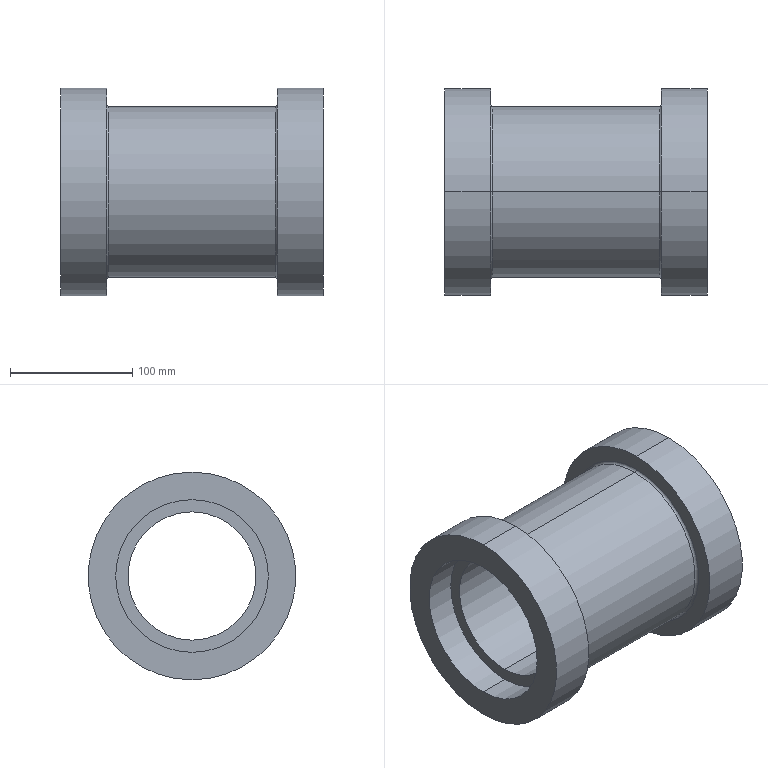Part | SolidWorks | features ICE 3, Cut 1, Extrusion 1, Fillet 1 | 1 solid | 22 faces | box 215 x 170 x 170 mm | volume 1815913 mm3 | cylinder 12 | plane 6 | torus 4 | commonest cylinder face diameters 125 x4 170 x4 105 x2 140 x2
STEP:
#1=CARTESIAN_POINT('',(25.,0.,-52.5));
#2=VERTEX_POINT('',#1);
#3=CARTESIAN_POINT('',(25.,0.,52.5));
#4=VERTEX_POINT('',#3);
#5=CARTESIAN_POINT('',(25.,0.,0.));
#6=DIRECTION('',(-1.,0.,0.));
#7=DIRECTION('',(0.,0.,1.));
#8=AXIS2_PLACEMENT_3D('',#5,#6,#7);
#9=CIRCLE('',#8,52.5);
#10=EDGE_CURVE('',#2,#4,#9,.T.);
#11=ORIENTED_EDGE('',*,*,#10,.T.);
#12=CARTESIAN_POINT('',(190.,0.,52.5));
#13=VERTEX_POINT('',#12);
#14=CARTESIAN_POINT('',(0.,0.,52.5));
#15=DIRECTION('',(1.,0.,0.));
#16=VECTOR('',#15,1000.);
#17=LINE('',#14,#16);
#18=EDGE_CURVE('',#4,#13,#17,.T.);
#19=ORIENTED_EDGE('',*,*,#18,.T.);
#20=CARTESIAN_POINT('',(190.,0.,-52.5));
#21=VERTEX_POINT('',#20);
#22=CARTESIAN_POINT('',(190.,0.,0.));
#23=DIRECTION('',(1.,0.,0.));
#24=DIRECTION('',(0.,0.,-1.));
#25=AXIS2_PLACEMENT_3D('',#22,#23,#24);
#26=CIRCLE('',#25,52.5);
#27=EDGE_CURVE('',#13,#21,#26,.T.);
#28=ORIENTED_EDGE('',*,*,#27,.T.);
#29=CARTESIAN_POINT('',(0.,0.,-52.5));
#30=DIRECTION('',(1.,0.,0.));
#31=VECTOR('',#30,1000.);
#32=LINE('',#29,#31);
#33=EDGE_CURVE('',#2,#21,#32,.T.);
#34=ORIENTED_EDGE('',*,*,#33,.F.);
#35=EDGE_LOOP('',(#11,#19,#28,#34));
#36=FACE_OUTER_BOUND('',#35,.T.);
#37=CARTESIAN_POINT('',(0.,0.,0.));
#38=DIRECTION('',(1.,0.,0.));
#39=DIRECTION('',(0.,0.,-1.));
#40=AXIS2_PLACEMENT_3D('',#37,#38,#39);
#41=CYLINDRICAL_SURFACE('',#40,52.5);
#42=ADVANCED_FACE('',(#36),#41,.F.);
#43=CARTESIAN_POINT('',(25.,0.,-62.5));
#44=VERTEX_POINT('',#43);
#45=CARTESIAN_POINT('',(25.,0.,62.5));
#46=VERTEX_POINT('',#45);
#47=CARTESIAN_POINT('',(25.,0.,0.));
#48=DIRECTION('',(-1.,0.,0.));
#49=DIRECTION('',(0.,0.,1.));
#50=AXIS2_PLACEMENT_3D('',#47,#48,#49);
#51=CIRCLE('',#50,62.5);
#52=EDGE_CURVE('',#44,#46,#51,.T.);
#53=ORIENTED_EDGE('',*,*,#52,.F.);
#54=CARTESIAN_POINT('',(0.,0.,-62.5));
#55=VERTEX_POINT('',#54);
#56=CARTESIAN_POINT('',(25.,0.,-62.5));
#57=DIRECTION('',(-1.,0.,0.));
#58=VECTOR('',#57,1000.);
#59=LINE('',#56,#58);
#60=EDGE_CURVE('',#44,#55,#59,.T.);
#61=ORIENTED_EDGE('',*,*,#60,.T.);
#62=CARTESIAN_POINT('',(0.,0.,62.5));
#63=VERTEX_POINT('',#62);
#64=CARTESIAN_POINT('',(0.,0.,0.));
#65=DIRECTION('',(-1.,0.,0.));
#66=DIRECTION('',(0.,0.,1.));
#67=AXIS2_PLACEMENT_3D('',#64,#65,#66);
#68=CIRCLE('',#67,62.5);
#69=EDGE_CURVE('',#55,#63,#68,.T.);
#70=ORIENTED_EDGE('',*,*,#69,.T.);
#71=CARTESIAN_POINT('',(25.,0.,62.5));
#72=DIRECTION('',(-1.,0.,0.));
#73=VECTOR('',#72,1000.);
#74=LINE('',#71,#73);
#75=EDGE_CURVE('',#46,#63,#74,.T.);
#76=ORIENTED_EDGE('',*,*,#75,.F.);
#77=EDGE_LOOP('',(#53,#61,#70,#76));
#78=FACE_OUTER_BOUND('',#77,.T.);
#79=CARTESIAN_POINT('',(25.,0.,0.));
#80=DIRECTION('',(-1.,0.,0.));
#81=DIRECTION('',(0.,0.,1.));
#82=AXIS2_PLACEMENT_3D('',#79,#80,#81);
#83=CYLINDRICAL_SURFACE('',#82,62.5);
#84=ADVANCED_FACE('',(#78),#83,.F.);
#85=CARTESIAN_POINT('',(190.,0.,62.5));
#86=VERTEX_POINT('',#85);
#87=CARTESIAN_POINT('',(190.,0.,-62.5));
#88=VERTEX_POINT('',#87);
#89=CARTESIAN_POINT('',(190.,0.,0.));
#90=DIRECTION('',(1.,0.,0.));
#91=DIRECTION('',(0.,0.,-1.));
#92=AXIS2_PLACEMENT_3D('',#89,#90,#91);
#93=CIRCLE('',#92,62.5);
#94=EDGE_CURVE('',#86,#88,#93,.T.);
#95=ORIENTED_EDGE('',*,*,#94,.F.);
#96=CARTESIAN_POINT('',(215.,0.,62.5));
#97=VERTEX_POINT('',#96);
#98=CARTESIAN_POINT('',(190.,0.,62.5));
#99=DIRECTION('',(1.,0.,0.));
#100=VECTOR('',#99,1000.);
#101=LINE('',#98,#100);
#102=EDGE_CURVE('',#86,#97,#101,.T.);
#103=ORIENTED_EDGE('',*,*,#102,.T.);
#104=CARTESIAN_POINT('',(215.,0.,-62.5));
#105=VERTEX_POINT('',#104);
#106=CARTESIAN_POINT('',(215.,0.,0.));
#107=DIRECTION('',(1.,0.,0.));
#108=DIRECTION('',(0.,0.,-1.));
#109=AXIS2_PLACEMENT_3D('',#106,#107,#108);
#110=CIRCLE('',#109,62.5);
#111=EDGE_CURVE('',#97,#105,#110,.T.);
#112=ORIENTED_EDGE('',*,*,#111,.T.);
#113=CARTESIAN_POINT('',(190.,0.,-62.5));
#114=DIRECTION('',(1.,0.,0.));
#115=VECTOR('',#114,1000.);
#116=LINE('',#113,#115);
#117=EDGE_CURVE('',#88,#105,#116,.T.);
#118=ORIENTED_EDGE('',*,*,#117,.F.);
#119=EDGE_LOOP('',(#95,#103,#112,#118));
#120=FACE_OUTER_BOUND('',#119,.T.);
#121=CARTESIAN_POINT('',(190.,0.,0.));
#122=DIRECTION('',(1.,0.,0.));
#123=DIRECTION('',(0.,0.,-1.));
#124=AXIS2_PLACEMENT_3D('',#121,#122,#123);
#125=CYLINDRICAL_SURFACE('',#124,62.5);
#126=ADVANCED_FACE('',(#120),#125,.F.);
#127=CARTESIAN_POINT('',(39.5,0.,70.));
#128=VERTEX_POINT('',#127);
#129=CARTESIAN_POINT('',(39.5,0.,-70.));
#130=VERTEX_POINT('',#129);
#131=CARTESIAN_POINT('',(39.5,0.,0.));
#132=DIRECTION('',(1.,0.,0.));
#133=DIRECTION('',(0.,0.,-1.));
#134=AXIS2_PLACEMENT_3D('',#131,#132,#133);
#135=CIRCLE('',#134,70.);
#136=EDGE_CURVE('',#128,#130,#135,.T.);
#137=ORIENTED_EDGE('',*,*,#136,.F.);
#138=CARTESIAN_POINT('',(37.5,0.,72.));
#139=VERTEX_POINT('',#138);
#140=CARTESIAN_POINT('',(39.5,0.,72.));
#141=DIRECTION('',(0.,1.,0.));
#142=DIRECTION('',(0.,0.,1.));
#143=AXIS2_PLACEMENT_3D('',#140,#141,#142);
#144=CIRCLE('',#143,2.);
#145=EDGE_CURVE('',#128,#139,#144,.T.);
#146=ORIENTED_EDGE('',*,*,#145,.T.);
#147=CARTESIAN_POINT('',(37.5,0.,-72.));
#148=VERTEX_POINT('',#147);
#149=CARTESIAN_POINT('',(37.5,0.,0.));
#150=DIRECTION('',(-1.,0.,0.));
#151=DIRECTION('',(0.,0.,-1.));
#152=AXIS2_PLACEMENT_3D('',#149,#150,#151);
#153=CIRCLE('',#152,72.);
#154=EDGE_CURVE('',#148,#139,#153,.T.);
#155=ORIENTED_EDGE('',*,*,#154,.F.);
#156=CARTESIAN_POINT('',(39.5,0.,-72.));
#157=DIRECTION('',(0.,-1.,0.));
#158=DIRECTION('',(0.,0.,-1.));
#159=AXIS2_PLACEMENT_3D('',#156,#157,#158);
#160=CIRCLE('',#159,2.);
#161=EDGE_CURVE('',#130,#148,#160,.T.);
#162=ORIENTED_EDGE('',*,*,#161,.F.);
#163=EDGE_LOOP('',(#137,#146,#155,#162));
#164=FACE_OUTER_BOUND('',#163,.T.);
#165=CARTESIAN_POINT('',(39.5,0.,0.));
#166=DIRECTION('',(1.,0.,0.));
#167=DIRECTION('',(0.,0.,-1.));
#168=AXIS2_PLACEMENT_3D('',#165,#166,#167);
#169=TOROIDAL_SURFACE('',#168,72.,2.);
#170=ADVANCED_FACE('',(#164),#169,.F.);
#171=CARTESIAN_POINT('',(177.5,0.,72.));
#172=VERTEX_POINT('',#171);
#173=CARTESIAN_POINT('',(177.5,0.,-72.));
#174=VERTEX_POINT('',#173);
#175=CARTESIAN_POINT('',(177.5,0.,0.));
#176=DIRECTION('',(1.,0.,0.));
#177=DIRECTION('',(0.,0.,-1.));
#178=AXIS2_PLACEMENT_3D('',#175,#176,#177);
#179=CIRCLE('',#178,72.);
#180=EDGE_CURVE('',#172,#174,#179,.T.);
#181=ORIENTED_EDGE('',*,*,#180,.F.);
#182=CARTESIAN_POINT('',(175.5,0.,70.));
#183=VERTEX_POINT('',#182);
#184=CARTESIAN_POINT('',(175.5,0.,72.));
#185=DIRECTION('',(0.,1.,0.));
#186=DIRECTION('',(0.,0.,1.));
#187=AXIS2_PLACEMENT_3D('',#184,#185,#186);
#188=CIRCLE('',#187,2.);
#189=EDGE_CURVE('',#172,#183,#188,.T.);
#190=ORIENTED_EDGE('',*,*,#189,.T.);
#191=CARTESIAN_POINT('',(175.5,0.,-70.));
#192=VERTEX_POINT('',#191);
#193=CARTESIAN_POINT('',(175.5,0.,0.));
#194=DIRECTION('',(-1.,0.,0.));
#195=DIRECTION('',(0.,0.,-1.));
#196=AXIS2_PLACEMENT_3D('',#193,#194,#195);
#197=CIRCLE('',#196,70.);
#198=EDGE_CURVE('',#192,#183,#197,.T.);
#199=ORIENTED_EDGE('',*,*,#198,.F.);
#200=CARTESIAN_POINT('',(175.5,0.,-72.));
#201=DIRECTION('',(0.,-1.,0.));
#202=DIRECTION('',(0.,0.,-1.));
#203=AXIS2_PLACEMENT_3D('',#200,#201,#202);
#204=CIRCLE('',#203,2.);
#205=EDGE_CURVE('',#174,#192,#204,.T.);
#206=ORIENTED_EDGE('',*,*,#205,.F.);
#207=EDGE_LOOP('',(#181,#190,#199,#206));
#208=FACE_OUTER_BOUND('',#207,.T.);
#209=CARTESIAN_POINT('',(175.5,0.,0.));
#210=DIRECTION('',(1.,0.,0.));
#211=DIRECTION('',(0.,0.,-1.));
#212=AXIS2_PLACEMENT_3D('',#209,#210,#211);
#213=TOROIDAL_SURFACE('',#212,72.,2.);
#214=ADVANCED_FACE('',(#208),#213,.F.);
#215=CARTESIAN_POINT('',(215.,0.,-85.));
#216=VERTEX_POINT('',#215);
#217=CARTESIAN_POINT('',(215.,0.,85.));
#218=VERTEX_POINT('',#217);
#219=CARTESIAN_POINT('',(215.,0.,0.));
#220=DIRECTION('',(1.,0.,0.));
#221=DIRECTION('',(0.,0.,-1.));
#222=AXIS2_PLACEMENT_3D('',#219,#220,#221);
#223=CIRCLE('',#222,85.);
#224=EDGE_CURVE('',#216,#218,#223,.T.);
#225=ORIENTED_EDGE('',*,*,#224,.F.);
#226=CARTESIAN_POINT('',(177.5,0.,-85.));
#227=VERTEX_POINT('',#226);
#228=CARTESIAN_POINT('',(215.,0.,-85.));
#229=DIRECTION('',(-1.,0.,0.));
#230=VECTOR('',#229,1000.);
#231=LINE('',#228,#230);
#232=EDGE_CURVE('',#216,#227,#231,.T.);
#233=ORIENTED_EDGE('',*,*,#232,.T.);
#234=CARTESIAN_POINT('',(177.5,0.,85.));
#235=VERTEX_POINT('',#234);
#236=CARTESIAN_POINT('',(177.5,0.,0.));
#237=DIRECTION('',(1.,0.,0.));
#238=DIRECTION('',(0.,0.,-1.));
#239=AXIS2_PLACEMENT_3D('',#236,#237,#238);
#240=CIRCLE('',#239,85.);
#241=EDGE_CURVE('',#227,#235,#240,.T.);
#242=ORIENTED_EDGE('',*,*,#241,.T.);
#243=CARTESIAN_POINT('',(215.,0.,85.));
#244=DIRECTION('',(-1.,0.,0.));
#245=VECTOR('',#244,1000.);
#246=LINE('',#243,#245);
#247=EDGE_CURVE('',#218,#235,#246,.T.);
#248=ORIENTED_EDGE('',*,*,#247,.F.);
#249=EDGE_LOOP('',(#225,#233,#242,#248));
#250=FACE_OUTER_BOUND('',#249,.T.);
#251=CARTESIAN_POINT('',(215.,0.,0.));
#252=DIRECTION('',(-1.,0.,0.));
#253=DIRECTION('',(0.,0.,1.));
#254=AXIS2_PLACEMENT_3D('',#251,#252,#253);
#255=CYLINDRICAL_SURFACE('',#254,85.);
#256=ADVANCED_FACE('',(#250),#255,.T.);
#257=CARTESIAN_POINT('',(39.5,0.,0.));
#258=DIRECTION('',(1.,0.,0.));
#259=DIRECTION('',(0.,0.,-1.));
#260=AXIS2_PLACEMENT_3D('',#257,#258,#259);
#261=CIRCLE('',#260,70.);
#262=EDGE_CURVE('',#130,#128,#261,.T.);
#263=ORIENTED_EDGE('',*,*,#262,.T.);
#264=CARTESIAN_POINT('',(37.5,0.,70.));
#265=DIRECTION('',(1.,0.,0.));
#266=VECTOR('',#265,1000.);
#267=LINE('',#264,#266);
#268=EDGE_CURVE('',#128,#183,#267,.T.);
#269=ORIENTED_EDGE('',*,*,#268,.T.);
#270=CARTESIAN_POINT('',(175.5,0.,0.));
#271=DIRECTION('',(-1.,0.,0.));
#272=DIRECTION('',(0.,0.,-1.));
#273=AXIS2_PLACEMENT_3D('',#270,#271,#272);
#274=CIRCLE('',#273,70.);
#275=EDGE_CURVE('',#183,#192,#274,.T.);
#276=ORIENTED_EDGE('',*,*,#275,.T.);
#277=CARTESIAN_POINT('',(37.5,0.,-70.));
#278=DIRECTION('',(1.,0.,0.));
#279=VECTOR('',#278,1000.);
#280=LINE('',#277,#279);
#281=EDGE_CURVE('',#130,#192,#280,.T.);
#282=ORIENTED_EDGE('',*,*,#281,.F.);
#283=EDGE_LOOP('',(#263,#269,#276,#282));
#284=FACE_OUTER_BOUND('',#283,.T.);
#285=CARTESIAN_POINT('',(37.5,0.,0.));
#286=DIRECTION('',(1.,0.,0.));
#287=DIRECTION('',(0.,0.,-1.));
#288=AXIS2_PLACEMENT_3D('',#285,#286,#287);
#289=CYLINDRICAL_SURFACE('',#288,70.);
#290=ADVANCED_FACE('',(#284),#289,.T.);
#291=CARTESIAN_POINT('',(37.5,0.,-85.));
#292=VERTEX_POINT('',#291);
#293=CARTESIAN_POINT('',(37.5,0.,85.));
#294=VERTEX_POINT('',#293);
#295=CARTESIAN_POINT('',(37.5,0.,0.));
#296=DIRECTION('',(1.,0.,0.));
#297=DIRECTION('',(0.,0.,-1.));
#298=AXIS2_PLACEMENT_3D('',#295,#296,#297);
#299=CIRCLE('',#298,85.);
#300=EDGE_CURVE('',#292,#294,#299,.T.);
#301=ORIENTED_EDGE('',*,*,#300,.F.);
#302=CARTESIAN_POINT('',(0.,0.,-85.));
#303=VERTEX_POINT('',#302);
#304=CARTESIAN_POINT('',(215.,0.,-85.));
#305=DIRECTION('',(-1.,0.,0.));
#306=VECTOR('',#305,1000.);
#307=LINE('',#304,#306);
#308=EDGE_CURVE('',#292,#303,#307,.T.);
#309=ORIENTED_EDGE('',*,*,#308,.T.);
#310=CARTESIAN_POINT('',(0.,0.,85.));
#311=VERTEX_POINT('',#310);
#312=CARTESIAN_POINT('',(0.,0.,0.));
#313=DIRECTION('',(1.,0.,0.));
#314=DIRECTION('',(0.,0.,-1.));
#315=AXIS2_PLACEMENT_3D('',#312,#313,#314);
#316=CIRCLE('',#315,85.);
#317=EDGE_CURVE('',#303,#311,#316,.T.);
#318=ORIENTED_EDGE('',*,*,#317,.T.);
#319=CARTESIAN_POINT('',(215.,0.,85.));
#320=DIRECTION('',(-1.,0.,0.));
#321=VECTOR('',#320,1000.);
#322=LINE('',#319,#321);
#323=EDGE_CURVE('',#294,#311,#322,.T.);
#324=ORIENTED_EDGE('',*,*,#323,.F.);
#325=EDGE_LOOP('',(#301,#309,#318,#324));
#326=FACE_OUTER_BOUND('',#325,.T.);
#327=CARTESIAN_POINT('',(215.,0.,0.));
#328=DIRECTION('',(-1.,0.,0.));
#329=DIRECTION('',(0.,0.,1.));
#330=AXIS2_PLACEMENT_3D('',#327,#328,#329);
#331=CYLINDRICAL_SURFACE('',#330,85.);
#332=ADVANCED_FACE('',(#326),#331,.T.);
#333=ORIENTED_EDGE('',*,*,#308,.F.);
#334=CARTESIAN_POINT('',(37.5,0.,0.));
#335=DIRECTION('',(1.,0.,0.));
#336=DIRECTION('',(0.,0.,-1.));
#337=AXIS2_PLACEMENT_3D('',#334,#335,#336);
#338=CIRCLE('',#337,85.);
#339=EDGE_CURVE('',#294,#292,#338,.T.);
#340=ORIENTED_EDGE('',*,*,#339,.F.);
#341=ORIENTED_EDGE('',*,*,#323,.T.);
#342=CARTESIAN_POINT('',(0.,0.,0.));
#343=DIRECTION('',(1.,0.,0.));
#344=DIRECTION('',(0.,0.,-1.));
#345=AXIS2_PLACEMENT_3D('',#342,#343,#344);
#346=CIRCLE('',#345,85.);
#347=EDGE_CURVE('',#311,#303,#346,.T.);
#348=ORIENTED_EDGE('',*,*,#347,.T.);
#349=EDGE_LOOP('',(#333,#340,#341,#348));
#350=FACE_OUTER_BOUND('',#349,.T.);
#351=CARTESIAN_POINT('',(215.,0.,0.));
#352=DIRECTION('',(-1.,0.,0.));
#353=DIRECTION('',(0.,0.,1.));
#354=AXIS2_PLACEMENT_3D('',#351,#352,#353);
#355=CYLINDRICAL_SURFACE('',#354,85.);
#356=ADVANCED_FACE('',(#350),#355,.T.);
#357=CARTESIAN_POINT('',(0.,0.,0.));
#358=DIRECTION('',(-1.,0.,0.));
#359=DIRECTION('',(0.,0.,1.));
#360=AXIS2_PLACEMENT_3D('',#357,#358,#359);
#361=CIRCLE('',#360,62.5);
#362=EDGE_CURVE('',#63,#55,#361,.T.);
#363=ORIENTED_EDGE('',*,*,#362,.F.);
#364=ORIENTED_EDGE('',*,*,#69,.F.);
#365=EDGE_LOOP('',(#363,#364));
#366=FACE_BOUND('',#365,.T.);
#367=ORIENTED_EDGE('',*,*,#347,.F.);
#368=ORIENTED_EDGE('',*,*,#317,.F.);
#369=EDGE_LOOP('',(#367,#368));
#370=FACE_OUTER_BOUND('',#369,.T.);
#371=CARTESIAN_POINT('',(0.,0.,0.));
#372=DIRECTION('',(1.,0.,0.));
#373=DIRECTION('',(0.,0.,-1.));
#374=AXIS2_PLACEMENT_3D('',#371,#372,#373);
#375=PLANE('',#374);
#376=ADVANCED_FACE('',(#366,#370),#375,.F.);
#377=ORIENTED_EDGE('',*,*,#154,.T.);
#378=CARTESIAN_POINT('',(37.5,0.,0.));
#379=DIRECTION('',(-1.,0.,0.));
#380=DIRECTION('',(0.,0.,-1.));
#381=AXIS2_PLACEMENT_3D('',#378,#379,#380);
#382=CIRCLE('',#381,72.);
#383=EDGE_CURVE('',#139,#148,#382,.T.);
#384=ORIENTED_EDGE('',*,*,#383,.T.);
#385=EDGE_LOOP('',(#377,#384));
#386=FACE_BOUND('',#385,.T.);
#387=ORIENTED_EDGE('',*,*,#339,.T.);
#388=ORIENTED_EDGE('',*,*,#300,.T.);
#389=EDGE_LOOP('',(#387,#388));
#390=FACE_OUTER_BOUND('',#389,.T.);
#391=CARTESIAN_POINT('',(37.5,0.,0.));
#392=DIRECTION('',(1.,0.,0.));
#393=DIRECTION('',(0.,0.,-1.));
#394=AXIS2_PLACEMENT_3D('',#391,#392,#393);
#395=PLANE('',#394);
#396=ADVANCED_FACE('',(#386,#390),#395,.T.);
#397=CARTESIAN_POINT('',(177.5,0.,0.));
#398=DIRECTION('',(1.,0.,0.));
#399=DIRECTION('',(0.,0.,-1.));
#400=AXIS2_PLACEMENT_3D('',#397,#398,#399);
#401=CIRCLE('',#400,72.);
#402=EDGE_CURVE('',#174,#172,#401,.T.);
#403=ORIENTED_EDGE('',*,*,#402,.T.);
#404=ORIENTED_EDGE('',*,*,#180,.T.);
#405=EDGE_LOOP('',(#403,#404));
#406=FACE_BOUND('',#405,.T.);
#407=CARTESIAN_POINT('',(177.5,0.,0.));
#408=DIRECTION('',(1.,0.,0.));
#409=DIRECTION('',(0.,0.,-1.));
#410=AXIS2_PLACEMENT_3D('',#407,#408,#409);
#411=CIRCLE('',#410,85.);
#412=EDGE_CURVE('',#235,#227,#411,.T.);
#413=ORIENTED_EDGE('',*,*,#412,.F.);
#414=ORIENTED_EDGE('',*,*,#241,.F.);
#415=EDGE_LOOP('',(#413,#414));
#416=FACE_OUTER_BOUND('',#415,.T.);
#417=CARTESIAN_POINT('',(177.5,0.,0.));
#418=DIRECTION('',(1.,0.,0.));
#419=DIRECTION('',(0.,0.,-1.));
#420=AXIS2_PLACEMENT_3D('',#417,#418,#419);
#421=PLANE('',#420);
#422=ADVANCED_FACE('',(#406,#416),#421,.F.);
#423=ORIENTED_EDGE('',*,*,#268,.F.);
#424=ORIENTED_EDGE('',*,*,#136,.T.);
#425=ORIENTED_EDGE('',*,*,#281,.T.);
#426=ORIENTED_EDGE('',*,*,#198,.T.);
#427=EDGE_LOOP('',(#423,#424,#425,#426));
#428=FACE_OUTER_BOUND('',#427,.T.);
#429=CARTESIAN_POINT('',(37.5,0.,0.));
#430=DIRECTION('',(1.,0.,0.));
#431=DIRECTION('',(0.,0.,-1.));
#432=AXIS2_PLACEMENT_3D('',#429,#430,#431);
#433=CYLINDRICAL_SURFACE('',#432,70.);
#434=ADVANCED_FACE('',(#428),#433,.T.);
#435=CARTESIAN_POINT('',(215.,0.,0.));
#436=DIRECTION('',(1.,0.,0.));
#437=DIRECTION('',(0.,0.,-1.));
#438=AXIS2_PLACEMENT_3D('',#435,#436,#437);
#439=CIRCLE('',#438,62.5);
#440=EDGE_CURVE('',#105,#97,#439,.T.);
#441=ORIENTED_EDGE('',*,*,#440,.F.);
#442=ORIENTED_EDGE('',*,*,#111,.F.);
#443=EDGE_LOOP('',(#441,#442));
#444=FACE_BOUND('',#443,.T.);
#445=CARTESIAN_POINT('',(215.,0.,0.));
#446=DIRECTION('',(1.,0.,0.));
#447=DIRECTION('',(0.,0.,-1.));
#448=AXIS2_PLACEMENT_3D('',#445,#446,#447);
#449=CIRCLE('',#448,85.);
#450=EDGE_CURVE('',#218,#216,#449,.T.);
#451=ORIENTED_EDGE('',*,*,#450,.T.);
#452=ORIENTED_EDGE('',*,*,#224,.T.);
#453=EDGE_LOOP('',(#451,#452));
#454=FACE_OUTER_BOUND('',#453,.T.);
#455=CARTESIAN_POINT('',(215.,0.,0.));
#456=DIRECTION('',(1.,0.,0.));
#457=DIRECTION('',(0.,0.,-1.));
#458=AXIS2_PLACEMENT_3D('',#455,#456,#457);
#459=PLANE('',#458);
#460=ADVANCED_FACE('',(#444,#454),#459,.T.);
#461=ORIENTED_EDGE('',*,*,#232,.F.);
#462=ORIENTED_EDGE('',*,*,#450,.F.);
#463=ORIENTED_EDGE('',*,*,#247,.T.);
#464=ORIENTED_EDGE('',*,*,#412,.T.);
#465=EDGE_LOOP('',(#461,#462,#463,#464));
#466=FACE_OUTER_BOUND('',#465,.T.);
#467=CARTESIAN_POINT('',(215.,0.,0.));
#468=DIRECTION('',(-1.,0.,0.));
#469=DIRECTION('',(0.,0.,1.));
#470=AXIS2_PLACEMENT_3D('',#467,#468,#469);
#471=CYLINDRICAL_SURFACE('',#470,85.);
#472=ADVANCED_FACE('',(#466),#471,.T.);
#473=ORIENTED_EDGE('',*,*,#189,.F.);
#474=ORIENTED_EDGE('',*,*,#402,.F.);
#475=ORIENTED_EDGE('',*,*,#205,.T.);
#476=ORIENTED_EDGE('',*,*,#275,.F.);
#477=EDGE_LOOP('',(#473,#474,#475,#476));
#478=FACE_OUTER_BOUND('',#477,.T.);
#479=CARTESIAN_POINT('',(175.5,0.,0.));
#480=DIRECTION('',(1.,0.,0.));
#481=DIRECTION('',(0.,0.,-1.));
#482=AXIS2_PLACEMENT_3D('',#479,#480,#481);
#483=TOROIDAL_SURFACE('',#482,72.,2.);
#484=ADVANCED_FACE('',(#478),#483,.F.);
#485=ORIENTED_EDGE('',*,*,#145,.F.);
#486=ORIENTED_EDGE('',*,*,#262,.F.);
#487=ORIENTED_EDGE('',*,*,#161,.T.);
#488=ORIENTED_EDGE('',*,*,#383,.F.);
#489=EDGE_LOOP('',(#485,#486,#487,#488));
#490=FACE_OUTER_BOUND('',#489,.T.);
#491=CARTESIAN_POINT('',(39.5,0.,0.));
#492=DIRECTION('',(1.,0.,0.));
#493=DIRECTION('',(0.,0.,-1.));
#494=AXIS2_PLACEMENT_3D('',#491,#492,#493);
#495=TOROIDAL_SURFACE('',#494,72.,2.);
#496=ADVANCED_FACE('',(#490),#495,.F.);
#497=ORIENTED_EDGE('',*,*,#102,.F.);
#498=CARTESIAN_POINT('',(190.,0.,0.));
#499=DIRECTION('',(1.,0.,0.));
#500=DIRECTION('',(0.,0.,-1.));
#501=AXIS2_PLACEMENT_3D('',#498,#499,#500);
#502=CIRCLE('',#501,62.5);
#503=EDGE_CURVE('',#88,#86,#502,.T.);
#504=ORIENTED_EDGE('',*,*,#503,.F.);
#505=ORIENTED_EDGE('',*,*,#117,.T.);
#506=ORIENTED_EDGE('',*,*,#440,.T.);
#507=EDGE_LOOP('',(#497,#504,#505,#506));
#508=FACE_OUTER_BOUND('',#507,.T.);
#509=CARTESIAN_POINT('',(190.,0.,0.));
#510=DIRECTION('',(1.,0.,0.));
#511=DIRECTION('',(0.,0.,-1.));
#512=AXIS2_PLACEMENT_3D('',#509,#510,#511);
#513=CYLINDRICAL_SURFACE('',#512,62.5);
#514=ADVANCED_FACE('',(#508),#513,.F.);
#515=CARTESIAN_POINT('',(190.,0.,0.));
#516=DIRECTION('',(1.,0.,0.));
#517=DIRECTION('',(0.,0.,-1.));
#518=AXIS2_PLACEMENT_3D('',#515,#516,#517);
#519=CIRCLE('',#518,52.5);
#520=EDGE_CURVE('',#21,#13,#519,.T.);
#521=ORIENTED_EDGE('',*,*,#520,.F.);
#522=ORIENTED_EDGE('',*,*,#27,.F.);
#523=EDGE_LOOP('',(#521,#522));
#524=FACE_BOUND('',#523,.T.);
#525=ORIENTED_EDGE('',*,*,#503,.T.);
#526=ORIENTED_EDGE('',*,*,#94,.T.);
#527=EDGE_LOOP('',(#525,#526));
#528=FACE_OUTER_BOUND('',#527,.T.);
#529=CARTESIAN_POINT('',(190.,0.,0.));
#530=DIRECTION('',(1.,0.,0.));
#531=DIRECTION('',(0.,0.,-1.));
#532=AXIS2_PLACEMENT_3D('',#529,#530,#531);
#533=PLANE('',#532);
#534=ADVANCED_FACE('',(#524,#528),#533,.T.);
#535=ORIENTED_EDGE('',*,*,#60,.F.);
#536=CARTESIAN_POINT('',(25.,0.,0.));
#537=DIRECTION('',(-1.,0.,0.));
#538=DIRECTION('',(0.,0.,1.));
#539=AXIS2_PLACEMENT_3D('',#536,#537,#538);
#540=CIRCLE('',#539,62.5);
#541=EDGE_CURVE('',#46,#44,#540,.T.);
#542=ORIENTED_EDGE('',*,*,#541,.F.);
#543=ORIENTED_EDGE('',*,*,#75,.T.);
#544=ORIENTED_EDGE('',*,*,#362,.T.);
#545=EDGE_LOOP('',(#535,#542,#543,#544));
#546=FACE_OUTER_BOUND('',#545,.T.);
#547=CARTESIAN_POINT('',(25.,0.,0.));
#548=DIRECTION('',(-1.,0.,0.));
#549=DIRECTION('',(0.,0.,1.));
#550=AXIS2_PLACEMENT_3D('',#547,#548,#549);
#551=CYLINDRICAL_SURFACE('',#550,62.5);
#552=ADVANCED_FACE('',(#546),#551,.F.);
#553=ORIENTED_EDGE('',*,*,#10,.F.);
#554=CARTESIAN_POINT('',(25.,0.,0.));
#555=DIRECTION('',(-1.,0.,0.));
#556=DIRECTION('',(0.,0.,1.));
#557=AXIS2_PLACEMENT_3D('',#554,#555,#556);
#558=CIRCLE('',#557,52.5);
#559=EDGE_CURVE('',#4,#2,#558,.T.);
#560=ORIENTED_EDGE('',*,*,#559,.F.);
#561=EDGE_LOOP('',(#553,#560));
#562=FACE_BOUND('',#561,.T.);
#563=ORIENTED_EDGE('',*,*,#541,.T.);
#564=ORIENTED_EDGE('',*,*,#52,.T.);
#565=EDGE_LOOP('',(#563,#564));
#566=FACE_OUTER_BOUND('',#565,.T.);
#567=CARTESIAN_POINT('',(25.,0.,0.));
#568=DIRECTION('',(-1.,0.,0.));
#569=DIRECTION('',(0.,0.,1.));
#570=AXIS2_PLACEMENT_3D('',#567,#568,#569);
#571=PLANE('',#570);
#572=ADVANCED_FACE('',(#562,#566),#571,.T.);
#573=ORIENTED_EDGE('',*,*,#18,.F.);
#574=ORIENTED_EDGE('',*,*,#559,.T.);
#575=ORIENTED_EDGE('',*,*,#33,.T.);
#576=ORIENTED_EDGE('',*,*,#520,.T.);
#577=EDGE_LOOP('',(#573,#574,#575,#576));
#578=FACE_OUTER_BOUND('',#577,.T.);
#579=CARTESIAN_POINT('',(0.,0.,0.));
#580=DIRECTION('',(1.,0.,0.));
#581=DIRECTION('',(0.,0.,-1.));
#582=AXIS2_PLACEMENT_3D('',#579,#580,#581);
#583=CYLINDRICAL_SURFACE('',#582,52.5);
#584=ADVANCED_FACE('',(#578),#583,.F.);
#585=CLOSED_SHELL('',(#42,#84,#126,#170,#214,#256,#290,#332,#356,#376,#396,#422,#434,#460,#472,#484,#496,#514,#534,#552,#572,#584));
#586=MANIFOLD_SOLID_BREP('',#585);
#587=CARTESIAN_POINT('',(0.,0.,0.));
#588=DIRECTION('',(0.,0.,1.));
#589=DIRECTION('',(1.,0.,0.));
#590=AXIS2_PLACEMENT_3D('',#587,#588,#589);
#591=(LENGTH_UNIT()NAMED_UNIT(*)SI_UNIT(.MILLI.,.METRE.));
#592=UNCERTAINTY_MEASURE_WITH_UNIT(LENGTH_MEASURE(0.00001),#591,'','');
#593=(NAMED_UNIT(*)PLANE_ANGLE_UNIT()SI_UNIT($,.RADIAN.));
#594=(NAMED_UNIT(*)SI_UNIT($,.STERADIAN.)SOLID_ANGLE_UNIT());
#595=(GEOMETRIC_REPRESENTATION_CONTEXT(3)GLOBAL_UNCERTAINTY_ASSIGNED_CONTEXT((#592))GLOBAL_UNIT_ASSIGNED_CONTEXT((#591,#593,#594))REPRESENTATION_CONTEXT('',''));
#596=ADVANCED_BREP_SHAPE_REPRESENTATION('',(#586,#590),#595);